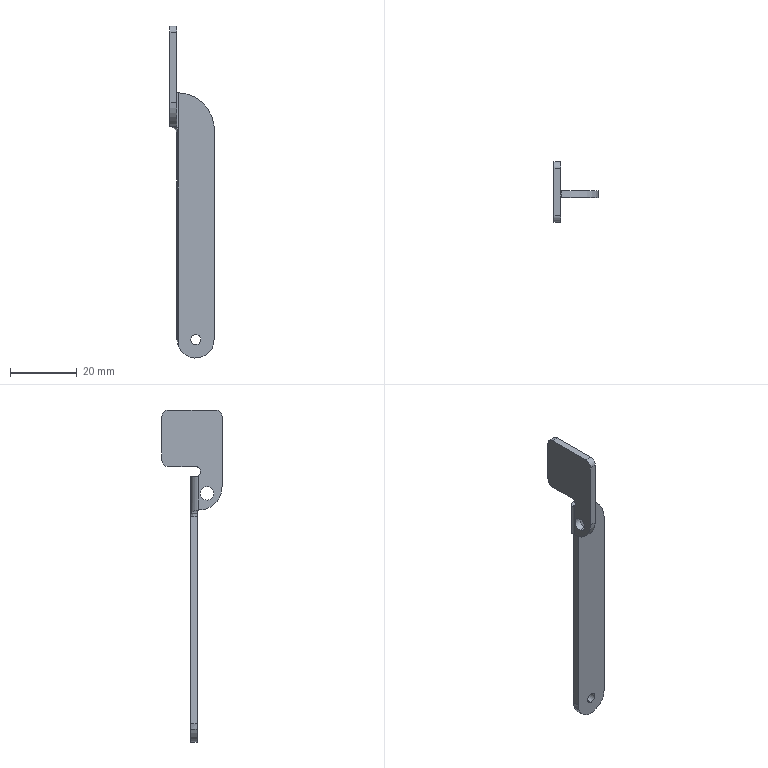Part | SolidWorks | features Fillet 4, HoleWzd 2, BaseBody 1, Draft 1, ICE 1 | 1 solid | 29 faces | box 13.227 x 18.048 x 99.5 mm | volume 2443 mm3 | cylinder 15 | plane 12 | spline 2 | commonest cylinder face diameters 4 x5 2 x2 3 x2 1 x1 3.447 x1 5 x1
STEP:
#1=CARTESIAN_POINT('',(-11.227,-4.964,107.));
#2=VERTEX_POINT('',#1);
#3=CARTESIAN_POINT('',(-11.227,-4.964,103.));
#4=VERTEX_POINT('',#3);
#5=CARTESIAN_POINT('',(-11.227,-4.964,105.));
#6=DIRECTION('',(1.,0.,0.));
#7=DIRECTION('',(0.,1.,0.));
#8=AXIS2_PLACEMENT_3D('',#5,#6,#7);
#9=CIRCLE('',#8,2.);
#10=EDGE_CURVE('',#2,#4,#9,.T.);
#11=ORIENTED_EDGE('',*,*,#10,.T.);
#12=CARTESIAN_POINT('',(-13.227,-4.964,103.));
#13=VERTEX_POINT('',#12);
#14=CARTESIAN_POINT('',(-13.227,-4.964,103.));
#15=DIRECTION('',(-1.,0.,0.));
#16=VECTOR('',#15,1000.);
#17=LINE('',#14,#16);
#18=EDGE_CURVE('',#4,#13,#17,.T.);
#19=ORIENTED_EDGE('',*,*,#18,.T.);
#20=CARTESIAN_POINT('',(-13.227,-4.964,107.));
#21=VERTEX_POINT('',#20);
#22=CARTESIAN_POINT('',(-13.227,-4.964,105.));
#23=DIRECTION('',(-1.,0.,0.));
#24=DIRECTION('',(0.,0.,1.));
#25=AXIS2_PLACEMENT_3D('',#22,#23,#24);
#26=CIRCLE('',#25,2.);
#27=EDGE_CURVE('',#13,#21,#26,.T.);
#28=ORIENTED_EDGE('',*,*,#27,.T.);
#29=CARTESIAN_POINT('',(-13.227,-4.964,107.));
#30=DIRECTION('',(-1.,0.,0.));
#31=VECTOR('',#30,1000.);
#32=LINE('',#29,#31);
#33=EDGE_CURVE('',#2,#21,#32,.T.);
#34=ORIENTED_EDGE('',*,*,#33,.F.);
#35=EDGE_LOOP('',(#11,#19,#28,#34));
#36=FACE_OUTER_BOUND('',#35,.T.);
#37=CARTESIAN_POINT('',(-13.227,-4.964,105.));
#38=DIRECTION('',(-1.,0.,0.));
#39=DIRECTION('',(0.,0.,1.));
#40=AXIS2_PLACEMENT_3D('',#37,#38,#39);
#41=CYLINDRICAL_SURFACE('',#40,2.);
#42=ADVANCED_FACE('',(#36),#41,.F.);
#43=CARTESIAN_POINT('',(-5.5,-2.,37.5));
#44=VERTEX_POINT('',#43);
#45=CARTESIAN_POINT('',(-5.5,-2.,34.5));
#46=VERTEX_POINT('',#45);
#47=CARTESIAN_POINT('',(-5.5,-2.,36.));
#48=DIRECTION('',(0.,-1.,0.));
#49=DIRECTION('',(0.,0.,-1.));
#50=AXIS2_PLACEMENT_3D('',#47,#48,#49);
#51=CIRCLE('',#50,1.5);
#52=EDGE_CURVE('',#44,#46,#51,.T.);
#53=ORIENTED_EDGE('',*,*,#52,.T.);
#54=CARTESIAN_POINT('',(-5.5,0.,34.5));
#55=VERTEX_POINT('',#54);
#56=CARTESIAN_POINT('',(-5.5,0.,34.5));
#57=DIRECTION('',(0.,1.,0.));
#58=VECTOR('',#57,1000.);
#59=LINE('',#56,#58);
#60=EDGE_CURVE('',#46,#55,#59,.T.);
#61=ORIENTED_EDGE('',*,*,#60,.T.);
#62=CARTESIAN_POINT('',(-5.5,0.,37.5));
#63=VERTEX_POINT('',#62);
#64=CARTESIAN_POINT('',(-5.5,0.,36.));
#65=DIRECTION('',(0.,1.,0.));
#66=DIRECTION('',(0.,0.,1.));
#67=AXIS2_PLACEMENT_3D('',#64,#65,#66);
#68=CIRCLE('',#67,1.5);
#69=EDGE_CURVE('',#55,#63,#68,.T.);
#70=ORIENTED_EDGE('',*,*,#69,.T.);
#71=CARTESIAN_POINT('',(-5.5,0.,37.5));
#72=DIRECTION('',(0.,1.,0.));
#73=VECTOR('',#72,1000.);
#74=LINE('',#71,#73);
#75=EDGE_CURVE('',#44,#63,#74,.T.);
#76=ORIENTED_EDGE('',*,*,#75,.F.);
#77=EDGE_LOOP('',(#53,#61,#70,#76));
#78=FACE_OUTER_BOUND('',#77,.T.);
#79=CARTESIAN_POINT('',(-5.5,0.,36.));
#80=DIRECTION('',(0.,1.,0.));
#81=DIRECTION('',(0.,0.,1.));
#82=AXIS2_PLACEMENT_3D('',#79,#80,#81);
#83=CYLINDRICAL_SURFACE('',#82,1.5);
#84=ADVANCED_FACE('',(#78),#83,.F.);
#85=ORIENTED_EDGE('',*,*,#10,.F.);
#86=CARTESIAN_POINT('',(-11.227,-4.964,105.));
#87=DIRECTION('',(1.,0.,0.));
#88=DIRECTION('',(0.,1.,0.));
#89=AXIS2_PLACEMENT_3D('',#86,#87,#88);
#90=CIRCLE('',#89,2.);
#91=EDGE_CURVE('',#4,#2,#90,.T.);
#92=ORIENTED_EDGE('',*,*,#91,.F.);
#93=EDGE_LOOP('',(#85,#92));
#94=FACE_BOUND('',#93,.T.);
#95=CARTESIAN_POINT('',(-11.227,-7.464,130.));
#96=VERTEX_POINT('',#95);
#97=CARTESIAN_POINT('',(-11.227,6.584,130.));
#98=VERTEX_POINT('',#97);
#99=CARTESIAN_POINT('',(-11.227,8.584,130.));
#100=DIRECTION('',(0.,1.,0.));
#101=VECTOR('',#100,1000.);
#102=LINE('',#99,#101);
#103=EDGE_CURVE('',#96,#98,#102,.T.);
#104=ORIENTED_EDGE('',*,*,#103,.F.);
#105=CARTESIAN_POINT('',(-11.227,-9.464,128.));
#106=VERTEX_POINT('',#105);
#107=CARTESIAN_POINT('',(-11.227,-7.464,128.));
#108=DIRECTION('',(1.,0.,0.));
#109=DIRECTION('',(0.,1.,0.));
#110=AXIS2_PLACEMENT_3D('',#107,#108,#109);
#111=CIRCLE('',#110,2.);
#112=EDGE_CURVE('',#96,#106,#111,.T.);
#113=ORIENTED_EDGE('',*,*,#112,.T.);
#114=CARTESIAN_POINT('',(-11.227,-9.464,107.));
#115=VERTEX_POINT('',#114);
#116=CARTESIAN_POINT('',(-11.227,-9.464,107.));
#117=DIRECTION('',(0.,0.,1.));
#118=VECTOR('',#117,1000.);
#119=LINE('',#116,#118);
#120=EDGE_CURVE('',#115,#106,#119,.T.);
#121=ORIENTED_EDGE('',*,*,#120,.F.);
#122=CARTESIAN_POINT('',(-11.227,-2.5,100.));
#123=VERTEX_POINT('',#122);
#124=CARTESIAN_POINT('',(-11.227,-2.464,107.));
#125=DIRECTION('',(-1.,0.,0.));
#126=DIRECTION('',(0.,0.,-1.));
#127=AXIS2_PLACEMENT_3D('',#124,#125,#126);
#128=CIRCLE('',#127,7.);
#129=EDGE_CURVE('',#123,#115,#128,.T.);
#130=ORIENTED_EDGE('',*,*,#129,.F.);
#131=CARTESIAN_POINT('',(-11.227,-2.5,110.));
#132=VERTEX_POINT('',#131);
#133=CARTESIAN_POINT('',(-11.227,-2.5,110.));
#134=DIRECTION('',(0.,0.,1.));
#135=VECTOR('',#134,1000.);
#136=LINE('',#133,#135);
#137=EDGE_CURVE('',#123,#132,#136,.T.);
#138=ORIENTED_EDGE('',*,*,#137,.T.);
#139=CARTESIAN_POINT('',(-11.227,-1.788,110.));
#140=VERTEX_POINT('',#139);
#141=CARTESIAN_POINT('',(-11.227,5.084,110.));
#142=DIRECTION('',(0.,1.,0.));
#143=VECTOR('',#142,1000.);
#144=LINE('',#141,#143);
#145=EDGE_CURVE('',#132,#140,#144,.T.);
#146=ORIENTED_EDGE('',*,*,#145,.T.);
#147=CARTESIAN_POINT('',(-11.227,-2.51,110.309));
#148=VERTEX_POINT('',#147);
#149=CARTESIAN_POINT('',(-11.227,-1.788,111.));
#150=DIRECTION('',(1.,0.,0.));
#151=DIRECTION('',(0.,0.,1.));
#152=AXIS2_PLACEMENT_3D('',#149,#150,#151);
#153=CIRCLE('',#152,1.);
#154=EDGE_CURVE('',#148,#140,#153,.T.);
#155=ORIENTED_EDGE('',*,*,#154,.F.);
#156=CARTESIAN_POINT('',(-11.227,-2.51,112.691));
#157=VERTEX_POINT('',#156);
#158=CARTESIAN_POINT('',(-11.227,-1.265,111.5));
#159=DIRECTION('',(1.,0.,0.));
#160=DIRECTION('',(0.,0.,-1.));
#161=AXIS2_PLACEMENT_3D('',#158,#159,#160);
#162=CIRCLE('',#161,1.723);
#163=EDGE_CURVE('',#157,#148,#162,.T.);
#164=ORIENTED_EDGE('',*,*,#163,.F.);
#165=CARTESIAN_POINT('',(-11.227,-1.788,113.));
#166=VERTEX_POINT('',#165);
#167=CARTESIAN_POINT('',(-11.227,-1.788,112.));
#168=DIRECTION('',(-1.,0.,0.));
#169=DIRECTION('',(0.,1.,0.));
#170=AXIS2_PLACEMENT_3D('',#167,#168,#169);
#171=CIRCLE('',#170,1.);
#172=EDGE_CURVE('',#157,#166,#171,.T.);
#173=ORIENTED_EDGE('',*,*,#172,.T.);
#174=CARTESIAN_POINT('',(-11.227,6.584,113.));
#175=VERTEX_POINT('',#174);
#176=CARTESIAN_POINT('',(-11.227,8.584,113.));
#177=DIRECTION('',(0.,1.,0.));
#178=VECTOR('',#177,1000.);
#179=LINE('',#176,#178);
#180=EDGE_CURVE('',#166,#175,#179,.T.);
#181=ORIENTED_EDGE('',*,*,#180,.T.);
#182=CARTESIAN_POINT('',(-11.227,8.584,115.));
#183=VERTEX_POINT('',#182);
#184=CARTESIAN_POINT('',(-11.227,6.584,115.));
#185=DIRECTION('',(1.,0.,0.));
#186=DIRECTION('',(0.,1.,0.));
#187=AXIS2_PLACEMENT_3D('',#184,#185,#186);
#188=CIRCLE('',#187,2.);
#189=EDGE_CURVE('',#175,#183,#188,.T.);
#190=ORIENTED_EDGE('',*,*,#189,.T.);
#191=CARTESIAN_POINT('',(-11.227,8.584,128.));
#192=VERTEX_POINT('',#191);
#193=CARTESIAN_POINT('',(-11.227,8.584,130.));
#194=DIRECTION('',(0.,0.,-1.));
#195=VECTOR('',#194,1000.);
#196=LINE('',#193,#195);
#197=EDGE_CURVE('',#192,#183,#196,.T.);
#198=ORIENTED_EDGE('',*,*,#197,.F.);
#199=CARTESIAN_POINT('',(-11.227,6.584,128.));
#200=DIRECTION('',(1.,0.,0.));
#201=DIRECTION('',(0.,1.,0.));
#202=AXIS2_PLACEMENT_3D('',#199,#200,#201);
#203=CIRCLE('',#202,2.);
#204=EDGE_CURVE('',#192,#98,#203,.T.);
#205=ORIENTED_EDGE('',*,*,#204,.T.);
#206=EDGE_LOOP('',(#104,#113,#121,#130,#138,#146,#155,#164,#173,#181,#190,#198,#205));
#207=FACE_OUTER_BOUND('',#206,.T.);
#208=CARTESIAN_POINT('',(-11.227,5.084,36.));
#209=DIRECTION('',(1.,0.,0.));
#210=DIRECTION('',(0.,0.,-1.));
#211=AXIS2_PLACEMENT_3D('',#208,#209,#210);
#212=PLANE('',#211);
#213=ADVANCED_FACE('',(#94,#207),#212,.T.);
#214=ORIENTED_EDGE('',*,*,#120,.T.);
#215=CARTESIAN_POINT('',(-13.227,-9.464,128.));
#216=VERTEX_POINT('',#215);
#217=CARTESIAN_POINT('',(-13.227,-9.464,128.));
#218=DIRECTION('',(-1.,0.,0.));
#219=VECTOR('',#218,1000.);
#220=LINE('',#217,#219);
#221=EDGE_CURVE('',#106,#216,#220,.T.);
#222=ORIENTED_EDGE('',*,*,#221,.T.);
#223=CARTESIAN_POINT('',(-13.227,-9.464,107.));
#224=VERTEX_POINT('',#223);
#225=CARTESIAN_POINT('',(-13.227,-9.464,107.));
#226=DIRECTION('',(0.,0.,1.));
#227=VECTOR('',#226,1000.);
#228=LINE('',#225,#227);
#229=EDGE_CURVE('',#224,#216,#228,.T.);
#230=ORIENTED_EDGE('',*,*,#229,.F.);
#231=CARTESIAN_POINT('',(-11.227,-9.464,107.));
#232=DIRECTION('',(-1.,0.,0.));
#233=VECTOR('',#232,1000.);
#234=LINE('',#231,#233);
#235=EDGE_CURVE('',#115,#224,#234,.T.);
#236=ORIENTED_EDGE('',*,*,#235,.F.);
#237=EDGE_LOOP('',(#214,#222,#230,#236));
#238=FACE_OUTER_BOUND('',#237,.T.);
#239=CARTESIAN_POINT('',(-11.227,-9.464,107.));
#240=DIRECTION('',(0.,-1.,0.));
#241=DIRECTION('',(0.,0.,1.));
#242=AXIS2_PLACEMENT_3D('',#239,#240,#241);
#243=PLANE('',#242);
#244=ADVANCED_FACE('',(#238),#243,.T.);
#245=CARTESIAN_POINT('',(-13.227,-4.964,105.));
#246=DIRECTION('',(-1.,0.,0.));
#247=DIRECTION('',(0.,0.,1.));
#248=AXIS2_PLACEMENT_3D('',#245,#246,#247);
#249=CIRCLE('',#248,2.);
#250=EDGE_CURVE('',#21,#13,#249,.T.);
#251=ORIENTED_EDGE('',*,*,#250,.F.);
#252=ORIENTED_EDGE('',*,*,#27,.F.);
#253=EDGE_LOOP('',(#251,#252));
#254=FACE_BOUND('',#253,.T.);
#255=CARTESIAN_POINT('',(-13.227,-2.51,110.309));
#256=VERTEX_POINT('',#255);
#257=CARTESIAN_POINT('',(-13.227,-2.5,110.298));
#258=VERTEX_POINT('',#257);
#259=CARTESIAN_POINT('',(-13.227,-1.788,111.));
#260=DIRECTION('',(1.,0.,0.));
#261=DIRECTION('',(0.,0.,1.));
#262=AXIS2_PLACEMENT_3D('',#259,#260,#261);
#263=CIRCLE('',#262,1.);
#264=EDGE_CURVE('',#256,#258,#263,.T.);
#265=ORIENTED_EDGE('',*,*,#264,.T.);
#266=CARTESIAN_POINT('',(-13.227,-2.5,100.));
#267=VERTEX_POINT('',#266);
#268=CARTESIAN_POINT('',(-13.227,-2.5,36.));
#269=DIRECTION('',(0.,0.,-1.));
#270=VECTOR('',#269,1000.);
#271=LINE('',#268,#270);
#272=EDGE_CURVE('',#258,#267,#271,.T.);
#273=ORIENTED_EDGE('',*,*,#272,.T.);
#274=CARTESIAN_POINT('',(-13.227,-2.464,107.));
#275=DIRECTION('',(-1.,0.,0.));
#276=DIRECTION('',(0.,0.,-1.));
#277=AXIS2_PLACEMENT_3D('',#274,#275,#276);
#278=CIRCLE('',#277,7.);
#279=EDGE_CURVE('',#267,#224,#278,.T.);
#280=ORIENTED_EDGE('',*,*,#279,.T.);
#281=ORIENTED_EDGE('',*,*,#229,.T.);
#282=CARTESIAN_POINT('',(-13.227,-7.464,130.));
#283=VERTEX_POINT('',#282);
#284=CARTESIAN_POINT('',(-13.227,-7.464,128.));
#285=DIRECTION('',(-1.,0.,0.));
#286=DIRECTION('',(0.,1.,0.));
#287=AXIS2_PLACEMENT_3D('',#284,#285,#286);
#288=CIRCLE('',#287,2.);
#289=EDGE_CURVE('',#216,#283,#288,.T.);
#290=ORIENTED_EDGE('',*,*,#289,.T.);
#291=CARTESIAN_POINT('',(-13.227,6.584,130.));
#292=VERTEX_POINT('',#291);
#293=CARTESIAN_POINT('',(-13.227,-9.464,130.));
#294=DIRECTION('',(0.,-1.,0.));
#295=VECTOR('',#294,1000.);
#296=LINE('',#293,#295);
#297=EDGE_CURVE('',#292,#283,#296,.T.);
#298=ORIENTED_EDGE('',*,*,#297,.F.);
#299=CARTESIAN_POINT('',(-13.227,8.584,128.));
#300=VERTEX_POINT('',#299);
#301=CARTESIAN_POINT('',(-13.227,6.584,128.));
#302=DIRECTION('',(-1.,0.,0.));
#303=DIRECTION('',(0.,1.,0.));
#304=AXIS2_PLACEMENT_3D('',#301,#302,#303);
#305=CIRCLE('',#304,2.);
#306=EDGE_CURVE('',#292,#300,#305,.T.);
#307=ORIENTED_EDGE('',*,*,#306,.T.);
#308=CARTESIAN_POINT('',(-13.227,8.584,115.));
#309=VERTEX_POINT('',#308);
#310=CARTESIAN_POINT('',(-13.227,8.584,130.));
#311=DIRECTION('',(0.,0.,-1.));
#312=VECTOR('',#311,1000.);
#313=LINE('',#310,#312);
#314=EDGE_CURVE('',#300,#309,#313,.T.);
#315=ORIENTED_EDGE('',*,*,#314,.T.);
#316=CARTESIAN_POINT('',(-13.227,6.584,113.));
#317=VERTEX_POINT('',#316);
#318=CARTESIAN_POINT('',(-13.227,6.584,115.));
#319=DIRECTION('',(-1.,0.,0.));
#320=DIRECTION('',(0.,1.,0.));
#321=AXIS2_PLACEMENT_3D('',#318,#319,#320);
#322=CIRCLE('',#321,2.);
#323=EDGE_CURVE('',#309,#317,#322,.T.);
#324=ORIENTED_EDGE('',*,*,#323,.T.);
#325=CARTESIAN_POINT('',(-13.227,-1.788,113.));
#326=VERTEX_POINT('',#325);
#327=CARTESIAN_POINT('',(-13.227,-9.464,113.));
#328=DIRECTION('',(0.,-1.,0.));
#329=VECTOR('',#328,1000.);
#330=LINE('',#327,#329);
#331=EDGE_CURVE('',#317,#326,#330,.T.);
#332=ORIENTED_EDGE('',*,*,#331,.T.);
#333=CARTESIAN_POINT('',(-13.227,-2.51,112.691));
#334=VERTEX_POINT('',#333);
#335=CARTESIAN_POINT('',(-13.227,-1.788,112.));
#336=DIRECTION('',(1.,0.,0.));
#337=DIRECTION('',(0.,1.,0.));
#338=AXIS2_PLACEMENT_3D('',#335,#336,#337);
#339=CIRCLE('',#338,1.);
#340=EDGE_CURVE('',#326,#334,#339,.T.);
#341=ORIENTED_EDGE('',*,*,#340,.T.);
#342=CARTESIAN_POINT('',(-13.227,-1.265,111.5));
#343=DIRECTION('',(1.,0.,0.));
#344=DIRECTION('',(0.,0.,-1.));
#345=AXIS2_PLACEMENT_3D('',#342,#343,#344);
#346=CIRCLE('',#345,1.723);
#347=EDGE_CURVE('',#334,#256,#346,.T.);
#348=ORIENTED_EDGE('',*,*,#347,.T.);
#349=EDGE_LOOP('',(#265,#273,#280,#281,#290,#298,#307,#315,#324,#332,#341,#348));
#350=FACE_OUTER_BOUND('',#349,.T.);
#351=CARTESIAN_POINT('',(-13.227,5.084,36.));
#352=DIRECTION('',(1.,0.,0.));
#353=DIRECTION('',(0.,0.,-1.));
#354=AXIS2_PLACEMENT_3D('',#351,#352,#353);
#355=PLANE('',#354);
#356=ADVANCED_FACE('',(#254,#350),#355,.F.);
#357=ORIENTED_EDGE('',*,*,#279,.F.);
#358=CARTESIAN_POINT('',(-13.227,-2.464,100.));
#359=VERTEX_POINT('',#358);
#360=CARTESIAN_POINT('',(-13.227,-2.5,100.));
#361=CARTESIAN_POINT('',(-13.227,-2.488,100.));
#362=CARTESIAN_POINT('',(-13.227,-2.476,100.));
#363=CARTESIAN_POINT('',(-13.227,-2.464,100.));
#364=B_SPLINE_CURVE_WITH_KNOTS('',3,(#360,#361,#362,#363),.UNSPECIFIED.,.F.,.F.,(4,4),(0.,0.00003574),.UNSPECIFIED.);
#365=EDGE_CURVE('',#267,#359,#364,.T.);
#366=ORIENTED_EDGE('',*,*,#365,.T.);
#367=CARTESIAN_POINT('',(-11.368,-2.464,100.));
#368=VERTEX_POINT('',#367);
#369=CARTESIAN_POINT('',(-12.227,-2.464,100.));
#370=DIRECTION('',(1.,0.,0.));
#371=VECTOR('',#370,1000.);
#372=LINE('',#369,#371);
#373=EDGE_CURVE('',#359,#368,#372,.T.);
#374=ORIENTED_EDGE('',*,*,#373,.T.);
#375=CARTESIAN_POINT('',(-11.227,-2.472,100.));
#376=VERTEX_POINT('',#375);
#377=CARTESIAN_POINT('',(-11.227,-2.472,100.));
#378=CARTESIAN_POINT('',(-11.368,-2.464,100.));
#379=B_SPLINE_CURVE_WITH_KNOTS('',1,(#377,#378),.UNSPECIFIED.,.F.,.F.,(2,2),(0.0003894,0.07058),.UNSPECIFIED.);
#380=EDGE_CURVE('',#376,#368,#379,.T.);
#381=ORIENTED_EDGE('',*,*,#380,.F.);
#382=CARTESIAN_POINT('',(-11.227,-2.472,100.));
#383=CARTESIAN_POINT('',(-11.227,-2.481,100.));
#384=CARTESIAN_POINT('',(-11.227,-2.491,100.));
#385=CARTESIAN_POINT('',(-11.227,-2.5,100.));
#386=B_SPLINE_CURVE_WITH_KNOTS('',3,(#382,#383,#384,#385),.UNSPECIFIED.,.F.,.F.,(4,4),(0.,0.00002787),.UNSPECIFIED.);
#387=EDGE_CURVE('',#376,#123,#386,.T.);
#388=ORIENTED_EDGE('',*,*,#387,.T.);
#389=ORIENTED_EDGE('',*,*,#129,.T.);
#390=ORIENTED_EDGE('',*,*,#235,.T.);
#391=EDGE_LOOP('',(#357,#366,#374,#381,#388,#389,#390));
#392=FACE_OUTER_BOUND('',#391,.T.);
#393=CARTESIAN_POINT('',(-11.227,-2.464,107.));
#394=DIRECTION('',(-1.,0.,0.));
#395=DIRECTION('',(0.,0.,1.));
#396=AXIS2_PLACEMENT_3D('',#393,#394,#395);
#397=CYLINDRICAL_SURFACE('',#396,7.);
#398=ADVANCED_FACE('',(#392),#397,.T.);
#399=CARTESIAN_POINT('',(-13.124,-1.788,110.));
#400=VERTEX_POINT('',#399);
#401=CARTESIAN_POINT('',(-12.227,-1.788,110.));
#402=DIRECTION('',(-1.,0.,0.));
#403=VECTOR('',#402,1000.);
#404=LINE('',#401,#403);
#405=EDGE_CURVE('',#140,#400,#404,.T.);
#406=ORIENTED_EDGE('',*,*,#405,.T.);
#407=CARTESIAN_POINT('',(-13.124,-1.788,110.));
#408=CARTESIAN_POINT('',(-13.162,-1.917,110.));
#409=CARTESIAN_POINT('',(-13.189,-2.048,110.025));
#410=CARTESIAN_POINT('',(-13.222,-2.292,110.126));
#411=CARTESIAN_POINT('',(-13.227,-2.405,110.202));
#412=CARTESIAN_POINT('',(-13.227,-2.5,110.298));
#413=B_SPLINE_CURVE_WITH_KNOTS('',3,(#407,#408,#409,#410,#411,#412),.UNSPECIFIED.,.F.,.F.,(4,2,4),(0.,0.0003988,0.0007976),.UNSPECIFIED.);
#414=EDGE_CURVE('',#400,#258,#413,.T.);
#415=ORIENTED_EDGE('',*,*,#414,.T.);
#416=ORIENTED_EDGE('',*,*,#264,.F.);
#417=CARTESIAN_POINT('',(-11.227,-2.51,110.309));
#418=DIRECTION('',(-1.,0.,0.));
#419=VECTOR('',#418,1000.);
#420=LINE('',#417,#419);
#421=EDGE_CURVE('',#148,#256,#420,.T.);
#422=ORIENTED_EDGE('',*,*,#421,.F.);
#423=ORIENTED_EDGE('',*,*,#154,.T.);
#424=EDGE_LOOP('',(#406,#415,#416,#422,#423));
#425=FACE_OUTER_BOUND('',#424,.T.);
#426=CARTESIAN_POINT('',(-11.227,-1.788,111.));
#427=DIRECTION('',(-1.,0.,0.));
#428=DIRECTION('',(0.,0.,1.));
#429=AXIS2_PLACEMENT_3D('',#426,#427,#428);
#430=CYLINDRICAL_SURFACE('',#429,1.);
#431=ADVANCED_FACE('',(#425),#430,.F.);
#432=ORIENTED_EDGE('',*,*,#347,.F.);
#433=CARTESIAN_POINT('',(-11.227,-2.51,112.691));
#434=DIRECTION('',(1.,0.,0.));
#435=VECTOR('',#434,1000.);
#436=LINE('',#433,#435);
#437=EDGE_CURVE('',#334,#157,#436,.T.);
#438=ORIENTED_EDGE('',*,*,#437,.T.);
#439=ORIENTED_EDGE('',*,*,#163,.T.);
#440=ORIENTED_EDGE('',*,*,#421,.T.);
#441=EDGE_LOOP('',(#432,#438,#439,#440));
#442=FACE_OUTER_BOUND('',#441,.T.);
#443=CARTESIAN_POINT('',(-11.227,-1.265,111.5));
#444=DIRECTION('',(-1.,0.,0.));
#445=DIRECTION('',(0.,0.,1.));
#446=AXIS2_PLACEMENT_3D('',#443,#444,#445);
#447=CYLINDRICAL_SURFACE('',#446,1.723);
#448=ADVANCED_FACE('',(#442),#447,.F.);
#449=CARTESIAN_POINT('',(0.,0.,100.));
#450=VERTEX_POINT('',#449);
#451=CARTESIAN_POINT('',(0.,0.,36.));
#452=VERTEX_POINT('',#451);
#453=CARTESIAN_POINT('',(0.,0.,100.));
#454=DIRECTION('',(0.,0.,-1.));
#455=VECTOR('',#454,1000.);
#456=LINE('',#453,#455);
#457=EDGE_CURVE('',#450,#452,#456,.T.);
#458=ORIENTED_EDGE('',*,*,#457,.F.);
#459=CARTESIAN_POINT('',(0.,-2.,100.));
#460=VERTEX_POINT('',#459);
#461=CARTESIAN_POINT('',(0.,-2.,100.));
#462=DIRECTION('',(0.,1.,0.));
#463=VECTOR('',#462,1000.);
#464=LINE('',#461,#463);
#465=EDGE_CURVE('',#460,#450,#464,.T.);
#466=ORIENTED_EDGE('',*,*,#465,.F.);
#467=CARTESIAN_POINT('',(0.,-2.,36.));
#468=VERTEX_POINT('',#467);
#469=CARTESIAN_POINT('',(0.,-2.,100.));
#470=DIRECTION('',(0.,0.,-1.));
#471=VECTOR('',#470,1000.);
#472=LINE('',#469,#471);
#473=EDGE_CURVE('',#460,#468,#472,.T.);
#474=ORIENTED_EDGE('',*,*,#473,.T.);
#475=CARTESIAN_POINT('',(0.,-2.,36.));
#476=DIRECTION('',(0.,1.,0.));
#477=VECTOR('',#476,1000.);
#478=LINE('',#475,#477);
#479=EDGE_CURVE('',#468,#452,#478,.T.);
#480=ORIENTED_EDGE('',*,*,#479,.T.);
#481=EDGE_LOOP('',(#458,#466,#474,#480));
#482=FACE_OUTER_BOUND('',#481,.T.);
#483=CARTESIAN_POINT('',(0.,-2.,100.));
#484=DIRECTION('',(1.,0.,0.));
#485=DIRECTION('',(0.,0.,-1.));
#486=AXIS2_PLACEMENT_3D('',#483,#484,#485);
#487=PLANE('',#486);
#488=ADVANCED_FACE('',(#482),#487,.T.);
#489=ORIENTED_EDGE('',*,*,#52,.F.);
#490=CARTESIAN_POINT('',(-5.5,-2.,36.));
#491=DIRECTION('',(0.,-1.,0.));
#492=DIRECTION('',(0.,0.,-1.));
#493=AXIS2_PLACEMENT_3D('',#490,#491,#492);
#494=CIRCLE('',#493,1.5);
#495=EDGE_CURVE('',#46,#44,#494,.T.);
#496=ORIENTED_EDGE('',*,*,#495,.F.);
#497=EDGE_LOOP('',(#489,#496));
#498=FACE_BOUND('',#497,.T.);
#499=CARTESIAN_POINT('',(-10.727,-2.,109.997));
#500=VERTEX_POINT('',#499);
#501=CARTESIAN_POINT('',(-11.,-2.,98.95));
#502=DIRECTION('',(0.,1.,0.));
#503=DIRECTION('',(0.,0.,1.));
#504=AXIS2_PLACEMENT_3D('',#501,#502,#503);
#505=CIRCLE('',#504,11.05);
#506=EDGE_CURVE('',#500,#460,#505,.T.);
#507=ORIENTED_EDGE('',*,*,#506,.F.);
#508=CARTESIAN_POINT('',(-10.727,-2.,34.29));
#509=VERTEX_POINT('',#508);
#510=CARTESIAN_POINT('',(-10.727,-2.,99.654));
#511=DIRECTION('',(0.,0.,-1.));
#512=VECTOR('',#511,1000.);
#513=LINE('',#510,#512);
#514=EDGE_CURVE('',#500,#509,#513,.T.);
#515=ORIENTED_EDGE('',*,*,#514,.T.);
#516=CARTESIAN_POINT('',(-5.5,-2.,36.));
#517=DIRECTION('',(0.,1.,0.));
#518=DIRECTION('',(0.,0.,-1.));
#519=AXIS2_PLACEMENT_3D('',#516,#517,#518);
#520=CIRCLE('',#519,5.5);
#521=EDGE_CURVE('',#468,#509,#520,.T.);
#522=ORIENTED_EDGE('',*,*,#521,.F.);
#523=ORIENTED_EDGE('',*,*,#473,.F.);
#524=EDGE_LOOP('',(#507,#515,#522,#523));
#525=FACE_OUTER_BOUND('',#524,.T.);
#526=CARTESIAN_POINT('',(-5.5,-2.,36.));
#527=DIRECTION('',(0.,-1.,0.));
#528=DIRECTION('',(0.,0.,-1.));
#529=AXIS2_PLACEMENT_3D('',#526,#527,#528);
#530=PLANE('',#529);
#531=ADVANCED_FACE('',(#498,#525),#530,.T.);
#532=CARTESIAN_POINT('',(-10.727,0.,34.29));
#533=VERTEX_POINT('',#532);
#534=CARTESIAN_POINT('',(-10.727,0.,34.29));
#535=CARTESIAN_POINT('',(-10.727,-2.,34.29));
#536=B_SPLINE_CURVE_WITH_KNOTS('',1,(#534,#535),.UNSPECIFIED.,.F.,.F.,(2,2),(0.,1.),.UNSPECIFIED.);
#537=EDGE_CURVE('',#533,#509,#536,.T.);
#538=ORIENTED_EDGE('',*,*,#537,.F.);
#539=CARTESIAN_POINT('',(-5.5,0.,36.));
#540=DIRECTION('',(0.,1.,0.));
#541=DIRECTION('',(0.,0.,-1.));
#542=AXIS2_PLACEMENT_3D('',#539,#540,#541);
#543=CIRCLE('',#542,5.5);
#544=EDGE_CURVE('',#452,#533,#543,.T.);
#545=ORIENTED_EDGE('',*,*,#544,.F.);
#546=ORIENTED_EDGE('',*,*,#479,.F.);
#547=ORIENTED_EDGE('',*,*,#521,.T.);
#548=EDGE_LOOP('',(#538,#545,#546,#547));
#549=FACE_OUTER_BOUND('',#548,.T.);
#550=CARTESIAN_POINT('',(-5.5,-2.,36.));
#551=DIRECTION('',(0.,1.,0.));
#552=DIRECTION('',(0.,0.,1.));
#553=AXIS2_PLACEMENT_3D('',#550,#551,#552);
#554=CYLINDRICAL_SURFACE('',#553,5.5);
#555=ADVANCED_FACE('',(#549),#554,.T.);
#556=CARTESIAN_POINT('',(-5.5,0.,36.));
#557=DIRECTION('',(0.,1.,0.));
#558=DIRECTION('',(0.,0.,1.));
#559=AXIS2_PLACEMENT_3D('',#556,#557,#558);
#560=CIRCLE('',#559,1.5);
#561=EDGE_CURVE('',#63,#55,#560,.T.);
#562=ORIENTED_EDGE('',*,*,#561,.F.);
#563=ORIENTED_EDGE('',*,*,#69,.F.);
#564=EDGE_LOOP('',(#562,#563));
#565=FACE_BOUND('',#564,.T.);
#566=ORIENTED_EDGE('',*,*,#544,.T.);
#567=CARTESIAN_POINT('',(-10.727,0.,109.997));
#568=VERTEX_POINT('',#567);
#569=CARTESIAN_POINT('',(-10.727,0.,36.));
#570=DIRECTION('',(0.,0.,1.));
#571=VECTOR('',#570,1000.);
#572=LINE('',#569,#571);
#573=EDGE_CURVE('',#533,#568,#572,.T.);
#574=ORIENTED_EDGE('',*,*,#573,.T.);
#575=CARTESIAN_POINT('',(-11.,0.,98.95));
#576=DIRECTION('',(0.,1.,0.));
#577=DIRECTION('',(0.,0.,1.));
#578=AXIS2_PLACEMENT_3D('',#575,#576,#577);
#579=CIRCLE('',#578,11.05);
#580=EDGE_CURVE('',#568,#450,#579,.T.);
#581=ORIENTED_EDGE('',*,*,#580,.T.);
#582=ORIENTED_EDGE('',*,*,#457,.T.);
#583=EDGE_LOOP('',(#566,#574,#581,#582));
#584=FACE_OUTER_BOUND('',#583,.T.);
#585=CARTESIAN_POINT('',(-5.5,0.,36.));
#586=DIRECTION('',(0.,-1.,0.));
#587=DIRECTION('',(0.,0.,-1.));
#588=AXIS2_PLACEMENT_3D('',#585,#586,#587);
#589=PLANE('',#588);
#590=ADVANCED_FACE('',(#565,#584),#589,.F.);
#591=ORIENTED_EDGE('',*,*,#580,.F.);
#592=CARTESIAN_POINT('',(-11.,-0.0149,110.));
#593=VERTEX_POINT('',#592);
#594=CARTESIAN_POINT('',(-10.727,0.,109.997));
#595=CARTESIAN_POINT('',(-10.819,0.,109.999));
#596=CARTESIAN_POINT('',(-10.909,-0.004965,110.));
#597=CARTESIAN_POINT('',(-11.,-0.0149,110.));
#598=B_SPLINE_CURVE_WITH_KNOTS('',3,(#594,#595,#596,#597),.UNSPECIFIED.,.F.,.F.,(4,4),(0.,0.000273),.UNSPECIFIED.);
#599=EDGE_CURVE('',#568,#593,#598,.T.);
#600=ORIENTED_EDGE('',*,*,#599,.T.);
#601=CARTESIAN_POINT('',(-11.,-2.081,110.));
#602=VERTEX_POINT('',#601);
#603=CARTESIAN_POINT('',(-11.,-2.,110.));
#604=DIRECTION('',(0.,-1.,0.));
#605=VECTOR('',#604,1000.);
#606=LINE('',#603,#605);
#607=EDGE_CURVE('',#593,#602,#606,.T.);
#608=ORIENTED_EDGE('',*,*,#607,.T.);
#609=CARTESIAN_POINT('',(-11.,-2.081,110.));
#610=CARTESIAN_POINT('',(-10.919,-2.028,110.));
#611=CARTESIAN_POINT('',(-10.824,-2.,109.999));
#612=CARTESIAN_POINT('',(-10.727,-2.,109.997));
#613=B_SPLINE_CURVE_WITH_KNOTS('',3,(#609,#610,#611,#612),.UNSPECIFIED.,.F.,.F.,(4,4),(0.,0.0002863),.UNSPECIFIED.);
#614=EDGE_CURVE('',#602,#500,#613,.T.);
#615=ORIENTED_EDGE('',*,*,#614,.T.);
#616=ORIENTED_EDGE('',*,*,#506,.T.);
#617=ORIENTED_EDGE('',*,*,#465,.T.);
#618=EDGE_LOOP('',(#591,#600,#608,#615,#616,#617));
#619=FACE_OUTER_BOUND('',#618,.T.);
#620=CARTESIAN_POINT('',(-11.,-2.,98.95));
#621=DIRECTION('',(0.,1.,0.));
#622=DIRECTION('',(0.,0.,1.));
#623=AXIS2_PLACEMENT_3D('',#620,#621,#622);
#624=CYLINDRICAL_SURFACE('',#623,11.05);
#625=ADVANCED_FACE('',(#619),#624,.T.);
#626=ORIENTED_EDGE('',*,*,#373,.F.);
#627=CARTESIAN_POINT('',(-13.224,-2.361,100.));
#628=VERTEX_POINT('',#627);
#629=CARTESIAN_POINT('',(-10.727,-2.5,100.));
#630=DIRECTION('',(0.,0.,-1.));
#631=DIRECTION('',(1.,0.,0.));
#632=AXIS2_PLACEMENT_3D('',#629,#630,#631);
#633=CIRCLE('',#632,2.5);
#634=EDGE_CURVE('',#359,#628,#633,.T.);
#635=ORIENTED_EDGE('',*,*,#634,.T.);
#636=CARTESIAN_POINT('',(-13.224,-2.361,100.));
#637=CARTESIAN_POINT('',(-12.605,-2.395,100.));
#638=CARTESIAN_POINT('',(-11.986,-2.43,100.));
#639=CARTESIAN_POINT('',(-11.368,-2.464,100.));
#640=B_SPLINE_CURVE_WITH_KNOTS('',3,(#636,#637,#638,#639),.UNSPECIFIED.,.F.,.F.,(4,4),(0.,0.9294),.UNSPECIFIED.);
#641=EDGE_CURVE('',#628,#368,#640,.T.);
#642=ORIENTED_EDGE('',*,*,#641,.T.);
#643=EDGE_LOOP('',(#626,#635,#642));
#644=FACE_OUTER_BOUND('',#643,.T.);
#645=CARTESIAN_POINT('',(-10.727,-2.5,100.));
#646=DIRECTION('',(0.,0.,1.));
#647=DIRECTION('',(1.,0.,0.));
#648=AXIS2_PLACEMENT_3D('',#645,#646,#647);
#649=PLANE('',#648);
#650=ADVANCED_FACE('',(#644),#649,.F.);
#651=ORIENTED_EDGE('',*,*,#641,.F.);
#652=CARTESIAN_POINT('',(-11.179,-0.04115,98.));
#653=VERTEX_POINT('',#652);
#654=CARTESIAN_POINT('',(-13.224,-2.361,100.));
#655=CARTESIAN_POINT('',(-13.214,-2.184,99.991));
#656=CARTESIAN_POINT('',(-13.186,-2.013,99.977));
#657=CARTESIAN_POINT('',(-13.095,-1.68,99.937));
#658=CARTESIAN_POINT('',(-13.033,-1.517,99.911));
#659=CARTESIAN_POINT('',(-12.876,-1.21,99.843));
#660=CARTESIAN_POINT('',(-12.783,-1.068,99.802));
#661=CARTESIAN_POINT('',(-12.574,-0.8064,99.699));
#662=CARTESIAN_POINT('',(-12.457,-0.6876,99.636));
#663=CARTESIAN_POINT('',(-12.215,-0.4846,99.487));
#664=CARTESIAN_POINT('',(-12.088,-0.3981,99.399));
#665=CARTESIAN_POINT('',(-11.841,-0.2572,99.192));
#666=CARTESIAN_POINT('',(-11.723,-0.2041,99.075));
#667=CARTESIAN_POINT('',(-11.511,-0.1232,98.808));
#668=CARTESIAN_POINT('',(-11.418,-0.09595,98.658));
#669=CARTESIAN_POINT('',(-11.271,-0.05867,98.342));
#670=CARTESIAN_POINT('',(-11.216,-0.04791,98.173));
#671=CARTESIAN_POINT('',(-11.179,-0.04115,98.));
#672=B_SPLINE_CURVE_WITH_KNOTS('',3,(#654,#655,#656,#657,#658,#659,#660,#661,#662,#663,#664,#665,#666,#667,#668,#669,#670,#671),.UNSPECIFIED.,.F.,.F.,(4,2,2,2,2,2,2,2,4),(0.,0.0005205,0.001041,0.001562,0.002082,0.002603,0.003123,0.003644,0.004164),.UNSPECIFIED.);
#673=EDGE_CURVE('',#628,#653,#672,.T.);
#674=ORIENTED_EDGE('',*,*,#673,.T.);
#675=CARTESIAN_POINT('',(-10.818,-2.008,98.));
#676=VERTEX_POINT('',#675);
#677=CARTESIAN_POINT('',(-11.179,-0.04115,98.));
#678=CARTESIAN_POINT('',(-10.818,-2.008,98.));
#679=B_SPLINE_CURVE_WITH_KNOTS('',1,(#677,#678),.UNSPECIFIED.,.F.,.F.,(2,2),(0.003495,0.005495),.UNSPECIFIED.);
#680=EDGE_CURVE('',#653,#676,#679,.T.);
#681=ORIENTED_EDGE('',*,*,#680,.T.);
#682=CARTESIAN_POINT('',(-10.818,-2.008,98.));
#683=CARTESIAN_POINT('',(-10.826,-2.01,98.184));
#684=CARTESIAN_POINT('',(-10.838,-2.012,98.368));
#685=CARTESIAN_POINT('',(-10.874,-2.022,98.733));
#686=CARTESIAN_POINT('',(-10.898,-2.029,98.916));
#687=CARTESIAN_POINT('',(-10.967,-2.059,99.277));
#688=CARTESIAN_POINT('',(-11.011,-2.081,99.455));
#689=CARTESIAN_POINT('',(-11.099,-2.163,99.706));
#690=CARTESIAN_POINT('',(-11.131,-2.199,99.786));
#691=CARTESIAN_POINT('',(-11.193,-2.308,99.922));
#692=CARTESIAN_POINT('',(-11.222,-2.382,99.976));
#693=CARTESIAN_POINT('',(-11.227,-2.472,100.));
#694=B_SPLINE_CURVE_WITH_KNOTS('',3,(#682,#683,#684,#685,#686,#687,#688,#689,#690,#691,#692,#693),.UNSPECIFIED.,.F.,.F.,(4,2,2,2,2,4),(0.,0.0005515,0.001103,0.001655,0.00193,0.002206),.UNSPECIFIED.);
#695=EDGE_CURVE('',#676,#376,#694,.T.);
#696=ORIENTED_EDGE('',*,*,#695,.T.);
#697=ORIENTED_EDGE('',*,*,#380,.T.);
#698=EDGE_LOOP('',(#651,#674,#681,#696,#697));
#699=FACE_OUTER_BOUND('',#698,.T.);
#700=CARTESIAN_POINT('',(-20.37,-1.962,100.));
#701=CARTESIAN_POINT('',(-20.264,-0.06482,99.974));
#702=CARTESIAN_POINT('',(-19.62,1.547,99.914));
#703=CARTESIAN_POINT('',(-17.999,4.026,99.721));
#704=CARTESIAN_POINT('',(-17.028,4.897,99.59));
#705=CARTESIAN_POINT('',(-15.25,6.1,99.257));
#706=CARTESIAN_POINT('',(-14.44,6.44,99.055));
#707=CARTESIAN_POINT('',(-13.18,6.864,98.58));
#708=CARTESIAN_POINT('',(-12.725,6.952,98.308));
#709=CARTESIAN_POINT('',(-12.472,6.998,98.));
#710=CARTESIAN_POINT('',(-18.49,-2.067,100.));
#711=CARTESIAN_POINT('',(-18.405,-0.5395,99.974));
#712=CARTESIAN_POINT('',(-17.887,0.7581,99.914));
#713=CARTESIAN_POINT('',(-16.581,2.754,99.721));
#714=CARTESIAN_POINT('',(-15.8,3.455,99.59));
#715=CARTESIAN_POINT('',(-14.369,4.424,99.257));
#716=CARTESIAN_POINT('',(-13.716,4.697,99.055));
#717=CARTESIAN_POINT('',(-12.702,5.039,98.58));
#718=CARTESIAN_POINT('',(-12.336,5.11,98.308));
#719=CARTESIAN_POINT('',(-12.132,5.147,98.));
#720=CARTESIAN_POINT('',(-17.044,-2.147,100.));
#721=CARTESIAN_POINT('',(-16.975,-0.9047,99.974));
#722=CARTESIAN_POINT('',(-16.553,0.1513,99.914));
#723=CARTESIAN_POINT('',(-15.491,1.775,99.721));
#724=CARTESIAN_POINT('',(-14.855,2.346,99.59));
#725=CARTESIAN_POINT('',(-13.691,3.134,99.257));
#726=CARTESIAN_POINT('',(-13.16,3.357,99.055));
#727=CARTESIAN_POINT('',(-12.334,3.635,98.58));
#728=CARTESIAN_POINT('',(-12.036,3.692,98.308));
#729=CARTESIAN_POINT('',(-11.871,3.723,98.));
#730=CARTESIAN_POINT('',(-15.932,-2.209,100.));
#731=CARTESIAN_POINT('',(-15.875,-1.186,99.974));
#732=CARTESIAN_POINT('',(-15.528,-0.3155,99.914));
#733=CARTESIAN_POINT('',(-14.652,1.023,99.721));
#734=CARTESIAN_POINT('',(-14.128,1.493,99.59));
#735=CARTESIAN_POINT('',(-13.169,2.142,99.257));
#736=CARTESIAN_POINT('',(-12.732,2.326,99.055));
#737=CARTESIAN_POINT('',(-12.051,2.555,98.58));
#738=CARTESIAN_POINT('',(-11.806,2.602,98.308));
#739=CARTESIAN_POINT('',(-11.669,2.627,98.));
#740=CARTESIAN_POINT('',(-15.077,-2.257,100.));
#741=CARTESIAN_POINT('',(-15.029,-1.402,99.974));
#742=CARTESIAN_POINT('',(-14.739,-0.6745,99.914));
#743=CARTESIAN_POINT('',(-14.007,0.4436,99.721));
#744=CARTESIAN_POINT('',(-13.569,0.8367,99.59));
#745=CARTESIAN_POINT('',(-12.768,1.379,99.257));
#746=CARTESIAN_POINT('',(-12.402,1.533,99.055));
#747=CARTESIAN_POINT('',(-11.834,1.724,98.58));
#748=CARTESIAN_POINT('',(-11.629,1.763,98.308));
#749=CARTESIAN_POINT('',(-11.515,1.784,98.));
#750=CARTESIAN_POINT('',(-14.419,-2.294,100.));
#751=CARTESIAN_POINT('',(-14.378,-1.568,99.974));
#752=CARTESIAN_POINT('',(-14.132,-0.9507,99.914));
#753=CARTESIAN_POINT('',(-13.511,-0.001747,99.721));
#754=CARTESIAN_POINT('',(-13.139,0.3319,99.59));
#755=CARTESIAN_POINT('',(-12.459,0.7922,99.257));
#756=CARTESIAN_POINT('',(-12.149,0.9224,99.055));
#757=CARTESIAN_POINT('',(-11.666,1.085,98.58));
#758=CARTESIAN_POINT('',(-11.492,1.118,98.308));
#759=CARTESIAN_POINT('',(-11.395,1.136,98.));
#760=CARTESIAN_POINT('',(-14.275,-2.302,100.));
#761=CARTESIAN_POINT('',(-14.237,-1.604,99.974));
#762=CARTESIAN_POINT('',(-14.,-1.011,99.914));
#763=CARTESIAN_POINT('',(-13.403,-0.09869,99.721));
#764=CARTESIAN_POINT('',(-13.046,0.222,99.59));
#765=CARTESIAN_POINT('',(-12.392,0.6645,99.257));
#766=CARTESIAN_POINT('',(-12.094,0.7896,99.055));
#767=CARTESIAN_POINT('',(-11.63,0.9458,98.58));
#768=CARTESIAN_POINT('',(-11.463,0.978,98.308));
#769=CARTESIAN_POINT('',(-11.37,0.9951,98.));
#770=CARTESIAN_POINT('',(-13.913,-2.322,100.));
#771=CARTESIAN_POINT('',(-13.878,-1.696,99.974));
#772=CARTESIAN_POINT('',(-13.665,-1.163,99.914));
#773=CARTESIAN_POINT('',(-13.129,-0.3444,99.721));
#774=CARTESIAN_POINT('',(-12.809,-0.0565,99.59));
#775=CARTESIAN_POINT('',(-12.221,0.3407,99.257));
#776=CARTESIAN_POINT('',(-11.954,0.453,99.055));
#777=CARTESIAN_POINT('',(-11.538,0.5932,98.58));
#778=CARTESIAN_POINT('',(-11.387,0.6222,98.308));
#779=CARTESIAN_POINT('',(-11.304,0.6375,98.));
#780=CARTESIAN_POINT('',(-13.523,-2.344,100.));
#781=CARTESIAN_POINT('',(-13.492,-1.794,99.974));
#782=CARTESIAN_POINT('',(-13.306,-1.327,99.914));
#783=CARTESIAN_POINT('',(-12.836,-0.6079,99.721));
#784=CARTESIAN_POINT('',(-12.554,-0.3552,99.59));
#785=CARTESIAN_POINT('',(-12.039,-0.006569,99.257));
#786=CARTESIAN_POINT('',(-11.804,0.092,99.055));
#787=CARTESIAN_POINT('',(-11.438,0.2151,98.58));
#788=CARTESIAN_POINT('',(-11.307,0.2405,98.308));
#789=CARTESIAN_POINT('',(-11.233,0.2539,98.));
#790=CARTESIAN_POINT('',(-13.224,-2.361,100.));
#791=CARTESIAN_POINT('',(-13.196,-1.87,99.974));
#792=CARTESIAN_POINT('',(-13.03,-1.452,99.914));
#793=CARTESIAN_POINT('',(-12.61,-0.8106,99.721));
#794=CARTESIAN_POINT('',(-12.358,-0.585,99.59));
#795=CARTESIAN_POINT('',(-11.898,-0.2737,99.257));
#796=CARTESIAN_POINT('',(-11.689,-0.1857,99.055));
#797=CARTESIAN_POINT('',(-11.362,-0.07583,98.58));
#798=CARTESIAN_POINT('',(-11.245,-0.05316,98.308));
#799=CARTESIAN_POINT('',(-11.179,-0.04115,98.));
#800=CARTESIAN_POINT('',(-11.227,-2.472,100.));
#801=CARTESIAN_POINT('',(-11.221,-2.374,99.974));
#802=CARTESIAN_POINT('',(-11.188,-2.29,99.914));
#803=CARTESIAN_POINT('',(-11.104,-2.162,99.721));
#804=CARTESIAN_POINT('',(-11.054,-2.117,99.59));
#805=CARTESIAN_POINT('',(-10.962,-2.055,99.257));
#806=CARTESIAN_POINT('',(-10.92,-2.037,99.055));
#807=CARTESIAN_POINT('',(-10.854,-2.015,98.58));
#808=CARTESIAN_POINT('',(-10.831,-2.011,98.308));
#809=CARTESIAN_POINT('',(-10.818,-2.008,98.));
#810=CARTESIAN_POINT('',(-10.927,-2.489,100.));
#811=CARTESIAN_POINT('',(-10.925,-2.45,99.974));
#812=CARTESIAN_POINT('',(-10.912,-2.416,99.914));
#813=CARTESIAN_POINT('',(-10.878,-2.365,99.721));
#814=CARTESIAN_POINT('',(-10.858,-2.347,99.59));
#815=CARTESIAN_POINT('',(-10.821,-2.322,99.257));
#816=CARTESIAN_POINT('',(-10.804,-2.315,99.055));
#817=CARTESIAN_POINT('',(-10.778,-2.306,98.58));
#818=CARTESIAN_POINT('',(-10.769,-2.304,98.308));
#819=CARTESIAN_POINT('',(-10.764,-2.303,98.));
#820=CARTESIAN_POINT('',(-10.538,-2.511,100.));
#821=CARTESIAN_POINT('',(-10.54,-2.548,99.974));
#822=CARTESIAN_POINT('',(-10.553,-2.58,99.914));
#823=CARTESIAN_POINT('',(-10.584,-2.628,99.721));
#824=CARTESIAN_POINT('',(-10.604,-2.646,99.59));
#825=CARTESIAN_POINT('',(-10.638,-2.669,99.257));
#826=CARTESIAN_POINT('',(-10.654,-2.676,99.055));
#827=CARTESIAN_POINT('',(-10.679,-2.684,98.58));
#828=CARTESIAN_POINT('',(-10.688,-2.686,98.308));
#829=CARTESIAN_POINT('',(-10.693,-2.687,98.));
#830=CARTESIAN_POINT('',(-10.032,-2.539,100.));
#831=CARTESIAN_POINT('',(-10.039,-2.676,99.974));
#832=CARTESIAN_POINT('',(-10.086,-2.792,99.914));
#833=CARTESIAN_POINT('',(-10.203,-2.971,99.721));
#834=CARTESIAN_POINT('',(-10.273,-3.034,99.59));
#835=CARTESIAN_POINT('',(-10.401,-3.121,99.257));
#836=CARTESIAN_POINT('',(-10.46,-3.145,99.055));
#837=CARTESIAN_POINT('',(-10.55,-3.176,98.58));
#838=CARTESIAN_POINT('',(-10.583,-3.182,98.308));
#839=CARTESIAN_POINT('',(-10.602,-3.186,98.));
#840=CARTESIAN_POINT('',(-9.373,-2.576,100.));
#841=CARTESIAN_POINT('',(-9.388,-2.842,99.974));
#842=CARTESIAN_POINT('',(-9.479,-3.068,99.914));
#843=CARTESIAN_POINT('',(-9.706,-3.416,99.721));
#844=CARTESIAN_POINT('',(-9.843,-3.539,99.59));
#845=CARTESIAN_POINT('',(-10.092,-3.708,99.257));
#846=CARTESIAN_POINT('',(-10.206,-3.755,99.055));
#847=CARTESIAN_POINT('',(-10.383,-3.815,98.58));
#848=CARTESIAN_POINT('',(-10.447,-3.827,98.308));
#849=CARTESIAN_POINT('',(-10.482,-3.834,98.));
#850=CARTESIAN_POINT('',(-8.518,-2.623,100.));
#851=CARTESIAN_POINT('',(-8.542,-3.058,99.974));
#852=CARTESIAN_POINT('',(-8.69,-3.427,99.914));
#853=CARTESIAN_POINT('',(-9.061,-3.995,99.721));
#854=CARTESIAN_POINT('',(-9.284,-4.195,99.59));
#855=CARTESIAN_POINT('',(-9.691,-4.471,99.257));
#856=CARTESIAN_POINT('',(-9.877,-4.549,99.055));
#857=CARTESIAN_POINT('',(-10.166,-4.646,98.58));
#858=CARTESIAN_POINT('',(-10.27,-4.666,98.308));
#859=CARTESIAN_POINT('',(-10.328,-4.677,98.));
#860=CARTESIAN_POINT('',(-7.406,-2.685,100.));
#861=CARTESIAN_POINT('',(-7.442,-3.339,99.974));
#862=CARTESIAN_POINT('',(-7.664,-3.894,99.914));
#863=CARTESIAN_POINT('',(-8.223,-4.748,99.721));
#864=CARTESIAN_POINT('',(-8.557,-5.048,99.59));
#865=CARTESIAN_POINT('',(-9.169,-5.463,99.257));
#866=CARTESIAN_POINT('',(-9.449,-5.58,99.055));
#867=CARTESIAN_POINT('',(-9.883,-5.726,98.58));
#868=CARTESIAN_POINT('',(-10.039,-5.756,98.308));
#869=CARTESIAN_POINT('',(-10.126,-5.772,98.));
#870=CARTESIAN_POINT('',(-5.96,-2.766,100.));
#871=CARTESIAN_POINT('',(-6.012,-3.704,99.974));
#872=CARTESIAN_POINT('',(-6.331,-4.501,99.914));
#873=CARTESIAN_POINT('',(-7.132,-5.727,99.721));
#874=CARTESIAN_POINT('',(-7.612,-6.157,99.59));
#875=CARTESIAN_POINT('',(-8.491,-6.752,99.257));
#876=CARTESIAN_POINT('',(-8.892,-6.92,99.055));
#877=CARTESIAN_POINT('',(-9.515,-7.13,98.58));
#878=CARTESIAN_POINT('',(-9.74,-7.173,98.308));
#879=CARTESIAN_POINT('',(-9.865,-7.196,98.));
#880=CARTESIAN_POINT('',(-4.081,-2.871,100.));
#881=CARTESIAN_POINT('',(-4.154,-4.179,99.974));
#882=CARTESIAN_POINT('',(-4.597,-5.29,99.914));
#883=CARTESIAN_POINT('',(-5.715,-6.999,99.721));
#884=CARTESIAN_POINT('',(-6.384,-7.599,99.59));
#885=CARTESIAN_POINT('',(-7.61,-8.428,99.257));
#886=CARTESIAN_POINT('',(-8.168,-8.663,99.055));
#887=CARTESIAN_POINT('',(-9.037,-8.955,98.58));
#888=CARTESIAN_POINT('',(-9.35,-9.016,98.308));
#889=CARTESIAN_POINT('',(-9.525,-9.048,98.));
#890=B_SPLINE_SURFACE_WITH_KNOTS('',1,3,((#700,#701,#702,#703,#704,#705,#706,#707,#708,#709),(#710,#711,#712,#713,#714,#715,#716,#717,#718,#719),(#720,#721,#722,#723,#724,#725,#726,#727,#728,#729),(#730,#731,#732,#733,#734,#735,#736,#737,#738,#739),(#740,#741,#742,#743,#744,#745,#746,#747,#748,#749),(#750,#751,#752,#753,#754,#755,#756,#757,#758,#759),(#760,#761,#762,#763,#764,#765,#766,#767,#768,#769),(#770,#771,#772,#773,#774,#775,#776,#777,#778,#779),(#780,#781,#782,#783,#784,#785,#786,#787,#788,#789),(#790,#791,#792,#793,#794,#795,#796,#797,#798,#799),(#800,#801,#802,#803,#804,#805,#806,#807,#808,#809),(#810,#811,#812,#813,#814,#815,#816,#817,#818,#819),(#820,#821,#822,#823,#824,#825,#826,#827,#828,#829),(#830,#831,#832,#833,#834,#835,#836,#837,#838,#839),(#840,#841,#842,#843,#844,#845,#846,#847,#848,#849),(#850,#851,#852,#853,#854,#855,#856,#857,#858,#859),(#860,#861,#862,#863,#864,#865,#866,#867,#868,#869),(#870,#871,#872,#873,#874,#875,#876,#877,#878,#879),(#880,#881,#882,#883,#884,#885,#886,#887,#888,#889)),.UNSPECIFIED.,.F.,.F.,.F.,(2,1,1,1,1,1,1,1,1,1,1,1,1,1,1,1,1,1,2),(4,2,2,2,4),(-3.579,-2.637,-1.913,-1.356,-0.9281,-0.5985,-0.5268,-0.345,-0.15,0.,1.,1.15,1.345,1.599,1.928,2.356,2.913,3.637,4.579),(0.,0.25,0.5,0.75,1.),.UNSPECIFIED.);
#891=ADVANCED_FACE('',(#699),#890,.F.);
#892=ORIENTED_EDGE('',*,*,#680,.F.);
#893=CARTESIAN_POINT('',(-11.179,-0.04115,36.));
#894=VERTEX_POINT('',#893);
#895=CARTESIAN_POINT('',(-11.179,-0.04115,98.));
#896=DIRECTION('',(0.,0.,-1.));
#897=VECTOR('',#896,1000.);
#898=LINE('',#895,#897);
#899=EDGE_CURVE('',#653,#894,#898,.T.);
#900=ORIENTED_EDGE('',*,*,#899,.T.);
#901=CARTESIAN_POINT('',(-10.818,-2.008,36.));
#902=VERTEX_POINT('',#901);
#903=CARTESIAN_POINT('',(-11.179,-0.04115,36.));
#904=CARTESIAN_POINT('',(-10.818,-2.008,36.));
#905=B_SPLINE_CURVE_WITH_KNOTS('',1,(#903,#904),.UNSPECIFIED.,.F.,.F.,(2,2),(0.00004184,0.002042),.UNSPECIFIED.);
#906=EDGE_CURVE('',#894,#902,#905,.T.);
#907=ORIENTED_EDGE('',*,*,#906,.T.);
#908=CARTESIAN_POINT('',(-10.818,-2.008,36.));
#909=DIRECTION('',(0.,0.,1.));
#910=VECTOR('',#909,1000.);
#911=LINE('',#908,#910);
#912=EDGE_CURVE('',#902,#676,#911,.T.);
#913=ORIENTED_EDGE('',*,*,#912,.T.);
#914=EDGE_LOOP('',(#892,#900,#907,#913));
#915=FACE_OUTER_BOUND('',#914,.T.);
#916=CARTESIAN_POINT('',(-11.187,0.,36.));
#917=DIRECTION('',(-0.9835,-0.1807,0.));
#918=DIRECTION('',(0.1807,-0.9835,0.));
#919=AXIS2_PLACEMENT_3D('',#916,#917,#918);
#920=PLANE('',#919);
#921=ADVANCED_FACE('',(#915),#920,.T.);
#922=ORIENTED_EDGE('',*,*,#906,.F.);
#923=CARTESIAN_POINT('',(-11.179,-0.04115,36.));
#924=CARTESIAN_POINT('',(-11.03,-0.01379,35.43));
#925=CARTESIAN_POINT('',(-10.879,0.,34.86));
#926=CARTESIAN_POINT('',(-10.727,0.,34.29));
#927=B_SPLINE_CURVE_WITH_KNOTS('',3,(#923,#924,#925,#926),.UNSPECIFIED.,.F.,.F.,(4,4),(0.,0.001769),.UNSPECIFIED.);
#928=EDGE_CURVE('',#894,#533,#927,.T.);
#929=ORIENTED_EDGE('',*,*,#928,.T.);
#930=ORIENTED_EDGE('',*,*,#537,.T.);
#931=CARTESIAN_POINT('',(-10.727,-2.,34.29));
#932=CARTESIAN_POINT('',(-10.745,-2.,34.623));
#933=CARTESIAN_POINT('',(-10.763,-2.001,34.956));
#934=CARTESIAN_POINT('',(-10.78,-2.003,35.289));
#935=CARTESIAN_POINT('',(-10.793,-2.004,35.526));
#936=CARTESIAN_POINT('',(-10.805,-2.006,35.763));
#937=CARTESIAN_POINT('',(-10.818,-2.008,36.));
#938=B_SPLINE_CURVE_WITH_KNOTS('',3,(#931,#932,#933,#934,#935,#936,#937),.UNSPECIFIED.,.F.,.F.,(4,3,4),(0.,0.001,0.001712),.UNSPECIFIED.);
#939=EDGE_CURVE('',#509,#902,#938,.T.);
#940=ORIENTED_EDGE('',*,*,#939,.T.);
#941=EDGE_LOOP('',(#922,#929,#930,#940));
#942=FACE_OUTER_BOUND('',#941,.T.);
#943=CARTESIAN_POINT('',(-12.965,-0.06419,41.917));
#944=CARTESIAN_POINT('',(-12.388,0.04185,39.945));
#945=CARTESIAN_POINT('',(-11.811,0.1479,37.972));
#946=CARTESIAN_POINT('',(-11.233,0.2539,36.));
#947=CARTESIAN_POINT('',(-11.067,0.2846,35.43));
#948=CARTESIAN_POINT('',(-10.897,0.3,34.86));
#949=CARTESIAN_POINT('',(-10.727,0.3,34.29));
#950=CARTESIAN_POINT('',(-12.725,-0.3252,41.917));
#951=CARTESIAN_POINT('',(-12.21,-0.2305,39.945));
#952=CARTESIAN_POINT('',(-11.695,-0.1358,37.972));
#953=CARTESIAN_POINT('',(-11.179,-0.04115,36.));
#954=CARTESIAN_POINT('',(-11.03,-0.01379,35.43));
#955=CARTESIAN_POINT('',(-10.879,0.,34.86));
#956=CARTESIAN_POINT('',(-10.727,0.,34.29));
#957=CARTESIAN_POINT('',(-11.127,-2.065,41.917));
#958=CARTESIAN_POINT('',(-11.024,-2.046,39.945));
#959=CARTESIAN_POINT('',(-10.921,-2.027,37.972));
#960=CARTESIAN_POINT('',(-10.818,-2.008,36.));
#961=CARTESIAN_POINT('',(-10.788,-2.003,35.43));
#962=CARTESIAN_POINT('',(-10.758,-2.,34.86));
#963=CARTESIAN_POINT('',(-10.727,-2.,34.29));
#964=CARTESIAN_POINT('',(-10.887,-2.326,41.917));
#965=CARTESIAN_POINT('',(-10.846,-2.318,39.945));
#966=CARTESIAN_POINT('',(-10.805,-2.311,37.972));
#967=CARTESIAN_POINT('',(-10.764,-2.303,36.));
#968=CARTESIAN_POINT('',(-10.752,-2.301,35.43));
#969=CARTESIAN_POINT('',(-10.74,-2.3,34.86));
#970=CARTESIAN_POINT('',(-10.727,-2.3,34.29));
#971=CARTESIAN_POINT('',(-10.727,-2.5,41.917));
#972=CARTESIAN_POINT('',(-10.727,-2.5,39.945));
#973=CARTESIAN_POINT('',(-10.727,-2.5,37.972));
#974=CARTESIAN_POINT('',(-10.727,-2.5,36.));
#975=CARTESIAN_POINT('',(-10.727,-2.5,35.43));
#976=CARTESIAN_POINT('',(-10.727,-2.5,34.86));
#977=CARTESIAN_POINT('',(-10.727,-2.5,34.29));
#978=B_SPLINE_SURFACE_WITH_KNOTS('',1,3,((#943,#944,#945,#946,#947,#948,#949),(#950,#951,#952,#953,#954,#955,#956),(#957,#958,#959,#960,#961,#962,#963),(#964,#965,#966,#967,#968,#969,#970),(#971,#972,#973,#974,#975,#976,#977)),.UNSPECIFIED.,.F.,.F.,.F.,(2,1,1,1,2),(4,3,4),(-0.15,0.,1.,1.15,1.25),(-3.461,0.,1.),.UNSPECIFIED.);
#979=ADVANCED_FACE('',(#942),#978,.F.);
#980=ORIENTED_EDGE('',*,*,#607,.F.);
#981=CARTESIAN_POINT('',(-10.727,-2.5,110.));
#982=DIRECTION('',(0.,0.,1.));
#983=DIRECTION('',(-1.,0.,0.));
#984=AXIS2_PLACEMENT_3D('',#981,#982,#983);
#985=CIRCLE('',#984,2.5);
#986=EDGE_CURVE('',#593,#400,#985,.T.);
#987=ORIENTED_EDGE('',*,*,#986,.T.);
#988=ORIENTED_EDGE('',*,*,#405,.F.);
#989=ORIENTED_EDGE('',*,*,#145,.F.);
#990=CARTESIAN_POINT('',(-10.727,-2.5,110.));
#991=DIRECTION('',(0.,0.,-1.));
#992=DIRECTION('',(-1.,0.,0.));
#993=AXIS2_PLACEMENT_3D('',#990,#991,#992);
#994=CIRCLE('',#993,0.5);
#995=EDGE_CURVE('',#132,#602,#994,.T.);
#996=ORIENTED_EDGE('',*,*,#995,.T.);
#997=EDGE_LOOP('',(#980,#987,#988,#989,#996));
#998=FACE_OUTER_BOUND('',#997,.T.);
#999=CARTESIAN_POINT('',(-10.727,-2.5,110.));
#1000=DIRECTION('',(0.,0.,-1.));
#1001=DIRECTION('',(-1.,0.,0.));
#1002=AXIS2_PLACEMENT_3D('',#999,#1000,#1001);
#1003=PLANE('',#1002);
#1004=ADVANCED_FACE('',(#998),#1003,.F.);
#1005=ORIENTED_EDGE('',*,*,#331,.F.);
#1006=CARTESIAN_POINT('',(-11.227,6.584,113.));
#1007=DIRECTION('',(1.,0.,0.));
#1008=VECTOR('',#1007,1000.);
#1009=LINE('',#1006,#1008);
#1010=EDGE_CURVE('',#317,#175,#1009,.T.);
#1011=ORIENTED_EDGE('',*,*,#1010,.T.);
#1012=ORIENTED_EDGE('',*,*,#180,.F.);
#1013=CARTESIAN_POINT('',(-13.227,-1.788,113.));
#1014=DIRECTION('',(-1.,0.,0.));
#1015=VECTOR('',#1014,1000.);
#1016=LINE('',#1013,#1015);
#1017=EDGE_CURVE('',#166,#326,#1016,.T.);
#1018=ORIENTED_EDGE('',*,*,#1017,.T.);
#1019=EDGE_LOOP('',(#1005,#1011,#1012,#1018));
#1020=FACE_OUTER_BOUND('',#1019,.T.);
#1021=CARTESIAN_POINT('',(0.,0.,113.));
#1022=DIRECTION('',(0.,0.,-1.));
#1023=DIRECTION('',(-1.,0.,0.));
#1024=AXIS2_PLACEMENT_3D('',#1021,#1022,#1023);
#1025=PLANE('',#1024);
#1026=ADVANCED_FACE('',(#1020),#1025,.T.);
#1027=ORIENTED_EDGE('',*,*,#197,.T.);
#1028=CARTESIAN_POINT('',(-13.227,8.584,115.));
#1029=DIRECTION('',(-1.,0.,0.));
#1030=VECTOR('',#1029,1000.);
#1031=LINE('',#1028,#1030);
#1032=EDGE_CURVE('',#183,#309,#1031,.T.);
#1033=ORIENTED_EDGE('',*,*,#1032,.T.);
#1034=ORIENTED_EDGE('',*,*,#314,.F.);
#1035=CARTESIAN_POINT('',(-13.227,8.584,128.));
#1036=DIRECTION('',(1.,0.,0.));
#1037=VECTOR('',#1036,1000.);
#1038=LINE('',#1035,#1037);
#1039=EDGE_CURVE('',#300,#192,#1038,.T.);
#1040=ORIENTED_EDGE('',*,*,#1039,.T.);
#1041=EDGE_LOOP('',(#1027,#1033,#1034,#1040));
#1042=FACE_OUTER_BOUND('',#1041,.T.);
#1043=CARTESIAN_POINT('',(-13.227,8.584,130.));
#1044=DIRECTION('',(0.,-1.,0.));
#1045=DIRECTION('',(1.,0.,0.));
#1046=AXIS2_PLACEMENT_3D('',#1043,#1044,#1045);
#1047=PLANE('',#1046);
#1048=ADVANCED_FACE('',(#1042),#1047,.F.);
#1049=ORIENTED_EDGE('',*,*,#297,.T.);
#1050=CARTESIAN_POINT('',(-11.227,-7.464,130.));
#1051=DIRECTION('',(1.,0.,0.));
#1052=VECTOR('',#1051,1000.);
#1053=LINE('',#1050,#1052);
#1054=EDGE_CURVE('',#283,#96,#1053,.T.);
#1055=ORIENTED_EDGE('',*,*,#1054,.T.);
#1056=ORIENTED_EDGE('',*,*,#103,.T.);
#1057=CARTESIAN_POINT('',(0.,6.584,130.));
#1058=DIRECTION('',(-1.,0.,0.));
#1059=VECTOR('',#1058,1000.);
#1060=LINE('',#1057,#1059);
#1061=EDGE_CURVE('',#98,#292,#1060,.T.);
#1062=ORIENTED_EDGE('',*,*,#1061,.T.);
#1063=EDGE_LOOP('',(#1049,#1055,#1056,#1062));
#1064=FACE_OUTER_BOUND('',#1063,.T.);
#1065=CARTESIAN_POINT('',(0.,0.,130.));
#1066=DIRECTION('',(0.,0.,-1.));
#1067=DIRECTION('',(-1.,0.,0.));
#1068=AXIS2_PLACEMENT_3D('',#1065,#1066,#1067);
#1069=PLANE('',#1068);
#1070=ADVANCED_FACE('',(#1064),#1069,.F.);
#1071=ORIENTED_EDGE('',*,*,#60,.F.);
#1072=ORIENTED_EDGE('',*,*,#495,.T.);
#1073=ORIENTED_EDGE('',*,*,#75,.T.);
#1074=ORIENTED_EDGE('',*,*,#561,.T.);
#1075=EDGE_LOOP('',(#1071,#1072,#1073,#1074));
#1076=FACE_OUTER_BOUND('',#1075,.T.);
#1077=CARTESIAN_POINT('',(-5.5,0.,36.));
#1078=DIRECTION('',(0.,1.,0.));
#1079=DIRECTION('',(0.,0.,1.));
#1080=AXIS2_PLACEMENT_3D('',#1077,#1078,#1079);
#1081=CYLINDRICAL_SURFACE('',#1080,1.5);
#1082=ADVANCED_FACE('',(#1076),#1081,.F.);
#1083=ORIENTED_EDGE('',*,*,#18,.F.);
#1084=ORIENTED_EDGE('',*,*,#91,.T.);
#1085=ORIENTED_EDGE('',*,*,#33,.T.);
#1086=ORIENTED_EDGE('',*,*,#250,.T.);
#1087=EDGE_LOOP('',(#1083,#1084,#1085,#1086));
#1088=FACE_OUTER_BOUND('',#1087,.T.);
#1089=CARTESIAN_POINT('',(-13.227,-4.964,105.));
#1090=DIRECTION('',(-1.,0.,0.));
#1091=DIRECTION('',(0.,0.,1.));
#1092=AXIS2_PLACEMENT_3D('',#1089,#1090,#1091);
#1093=CYLINDRICAL_SURFACE('',#1092,2.);
#1094=ADVANCED_FACE('',(#1088),#1093,.F.);
#1095=ORIENTED_EDGE('',*,*,#939,.F.);
#1096=ORIENTED_EDGE('',*,*,#514,.F.);
#1097=ORIENTED_EDGE('',*,*,#614,.F.);
#1098=ORIENTED_EDGE('',*,*,#995,.F.);
#1099=ORIENTED_EDGE('',*,*,#137,.F.);
#1100=ORIENTED_EDGE('',*,*,#387,.F.);
#1101=ORIENTED_EDGE('',*,*,#695,.F.);
#1102=ORIENTED_EDGE('',*,*,#912,.F.);
#1103=EDGE_LOOP('',(#1095,#1096,#1097,#1098,#1099,#1100,#1101,#1102));
#1104=FACE_OUTER_BOUND('',#1103,.T.);
#1105=CARTESIAN_POINT('',(-10.727,-2.5,36.));
#1106=DIRECTION('',(0.,0.,-1.));
#1107=DIRECTION('',(-1.,0.,0.));
#1108=AXIS2_PLACEMENT_3D('',#1105,#1106,#1107);
#1109=CYLINDRICAL_SURFACE('',#1108,0.5);
#1110=ADVANCED_FACE('',(#1104),#1109,.F.);
#1111=ORIENTED_EDGE('',*,*,#340,.F.);
#1112=ORIENTED_EDGE('',*,*,#1017,.F.);
#1113=ORIENTED_EDGE('',*,*,#172,.F.);
#1114=ORIENTED_EDGE('',*,*,#437,.F.);
#1115=EDGE_LOOP('',(#1111,#1112,#1113,#1114));
#1116=FACE_OUTER_BOUND('',#1115,.T.);
#1117=CARTESIAN_POINT('',(-11.227,-1.788,112.));
#1118=DIRECTION('',(-1.,0.,0.));
#1119=DIRECTION('',(0.,-1.,0.));
#1120=AXIS2_PLACEMENT_3D('',#1117,#1118,#1119);
#1121=CYLINDRICAL_SURFACE('',#1120,1.);
#1122=ADVANCED_FACE('',(#1116),#1121,.F.);
#1123=ORIENTED_EDGE('',*,*,#289,.F.);
#1124=ORIENTED_EDGE('',*,*,#221,.F.);
#1125=ORIENTED_EDGE('',*,*,#112,.F.);
#1126=ORIENTED_EDGE('',*,*,#1054,.F.);
#1127=EDGE_LOOP('',(#1123,#1124,#1125,#1126));
#1128=FACE_OUTER_BOUND('',#1127,.T.);
#1129=CARTESIAN_POINT('',(0.,-7.464,128.));
#1130=DIRECTION('',(-1.,0.,0.));
#1131=DIRECTION('',(0.,-1.,0.));
#1132=AXIS2_PLACEMENT_3D('',#1129,#1130,#1131);
#1133=CYLINDRICAL_SURFACE('',#1132,2.);
#1134=ADVANCED_FACE('',(#1128),#1133,.T.);
#1135=ORIENTED_EDGE('',*,*,#189,.F.);
#1136=ORIENTED_EDGE('',*,*,#1010,.F.);
#1137=ORIENTED_EDGE('',*,*,#323,.F.);
#1138=ORIENTED_EDGE('',*,*,#1032,.F.);
#1139=EDGE_LOOP('',(#1135,#1136,#1137,#1138));
#1140=FACE_OUTER_BOUND('',#1139,.T.);
#1141=CARTESIAN_POINT('',(-13.227,6.584,115.));
#1142=DIRECTION('',(1.,0.,0.));
#1143=DIRECTION('',(0.,1.,0.));
#1144=AXIS2_PLACEMENT_3D('',#1141,#1142,#1143);
#1145=CYLINDRICAL_SURFACE('',#1144,2.);
#1146=ADVANCED_FACE('',(#1140),#1145,.T.);
#1147=ORIENTED_EDGE('',*,*,#204,.F.);
#1148=ORIENTED_EDGE('',*,*,#1039,.F.);
#1149=ORIENTED_EDGE('',*,*,#306,.F.);
#1150=ORIENTED_EDGE('',*,*,#1061,.F.);
#1151=EDGE_LOOP('',(#1147,#1148,#1149,#1150));
#1152=FACE_OUTER_BOUND('',#1151,.T.);
#1153=CARTESIAN_POINT('',(0.,6.584,128.));
#1154=DIRECTION('',(-1.,0.,0.));
#1155=DIRECTION('',(0.,-1.,0.));
#1156=AXIS2_PLACEMENT_3D('',#1153,#1154,#1155);
#1157=CYLINDRICAL_SURFACE('',#1156,2.);
#1158=ADVANCED_FACE('',(#1152),#1157,.T.);
#1159=ORIENTED_EDGE('',*,*,#365,.F.);
#1160=ORIENTED_EDGE('',*,*,#272,.F.);
#1161=ORIENTED_EDGE('',*,*,#414,.F.);
#1162=ORIENTED_EDGE('',*,*,#986,.F.);
#1163=ORIENTED_EDGE('',*,*,#599,.F.);
#1164=ORIENTED_EDGE('',*,*,#573,.F.);
#1165=ORIENTED_EDGE('',*,*,#928,.F.);
#1166=ORIENTED_EDGE('',*,*,#899,.F.);
#1167=ORIENTED_EDGE('',*,*,#673,.F.);
#1168=ORIENTED_EDGE('',*,*,#634,.F.);
#1169=EDGE_LOOP('',(#1159,#1160,#1161,#1162,#1163,#1164,#1165,#1166,#1167,#1168));
#1170=FACE_OUTER_BOUND('',#1169,.T.);
#1171=CARTESIAN_POINT('',(-10.727,-2.5,36.));
#1172=DIRECTION('',(0.,0.,1.));
#1173=DIRECTION('',(1.,0.,0.));
#1174=AXIS2_PLACEMENT_3D('',#1171,#1172,#1173);
#1175=CYLINDRICAL_SURFACE('',#1174,2.5);
#1176=ADVANCED_FACE('',(#1170),#1175,.T.);
#1177=CLOSED_SHELL('',(#42,#84,#213,#244,#356,#398,#431,#448,#488,#531,#555,#590,#625,#650,#891,#921,#979,#1004,#1026,#1048,#1070,#1082,#1094,#1110,#1122,#1134,#1146,#1158,#1176));
#1178=MANIFOLD_SOLID_BREP('',#1177);
#1179=CARTESIAN_POINT('',(0.,0.,0.));
#1180=DIRECTION('',(0.,0.,1.));
#1181=DIRECTION('',(1.,0.,0.));
#1182=AXIS2_PLACEMENT_3D('',#1179,#1180,#1181);
#1183=(LENGTH_UNIT()NAMED_UNIT(*)SI_UNIT(.MILLI.,.METRE.));
#1184=UNCERTAINTY_MEASURE_WITH_UNIT(LENGTH_MEASURE(0.00001),#1183,'','');
#1185=(NAMED_UNIT(*)PLANE_ANGLE_UNIT()SI_UNIT($,.RADIAN.));
#1186=(NAMED_UNIT(*)SI_UNIT($,.STERADIAN.)SOLID_ANGLE_UNIT());
#1187=(GEOMETRIC_REPRESENTATION_CONTEXT(3)GLOBAL_UNCERTAINTY_ASSIGNED_CONTEXT((#1184))GLOBAL_UNIT_ASSIGNED_CONTEXT((#1183,#1185,#1186))REPRESENTATION_CONTEXT('',''));
#1188=ADVANCED_BREP_SHAPE_REPRESENTATION('',(#1178,#1182),#1187);